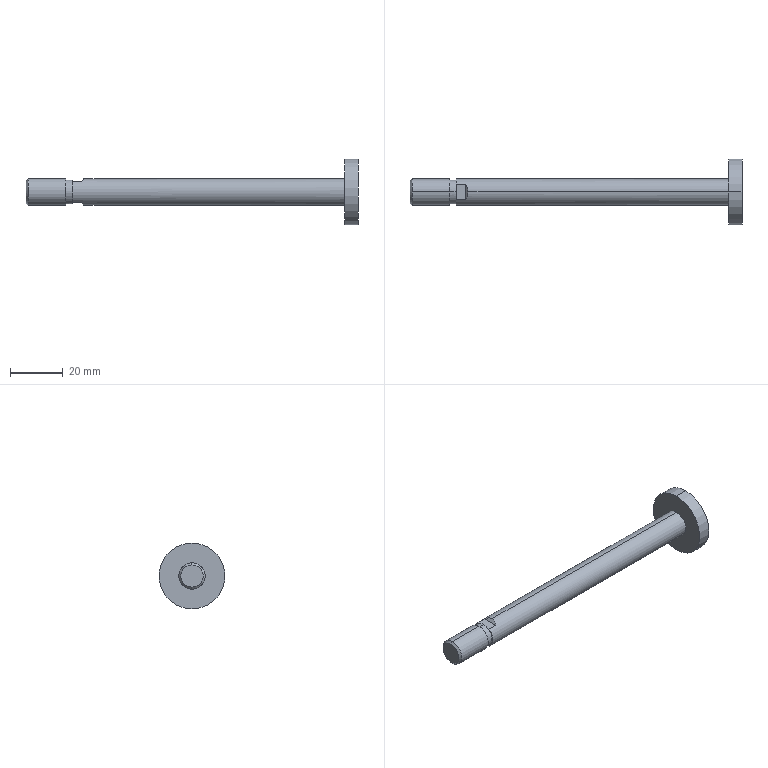Part | SolidWorks | features BaseBody 1 | 1 solid | 22 faces | box 126 x 25 x 25 mm | volume 11883 mm3 | plane 12 | cylinder 8 | cone 2 | commonest cylinder face diameters 10 x4 9.1 x2 25 x2
STEP:
#1=CARTESIAN_POINT('',(21.,3.,4.));
#2=VERTEX_POINT('',#1);
#3=CARTESIAN_POINT('',(22.,0.,5.));
#4=VERTEX_POINT('',#3);
#5=CARTESIAN_POINT('',(21.,3.,4.));
#6=CARTESIAN_POINT('',(21.655,2.127,4.655));
#7=CARTESIAN_POINT('',(22.,1.091,5.));
#8=CARTESIAN_POINT('',(22.,0.,5.));
#9=(BOUNDED_CURVE()B_SPLINE_CURVE(3,(#5,#6,#7,#8),.UNSPECIFIED.,.F.,.T.)B_SPLINE_CURVE_WITH_KNOTS((4,4),(5.64,6.283),.UNSPECIFIED.)CURVE()GEOMETRIC_REPRESENTATION_ITEM()RATIONAL_B_SPLINE_CURVE((1.,0.9658,0.9658,1.))REPRESENTATION_ITEM(''));
#10=EDGE_CURVE('',#2,#4,#9,.T.);
#11=ORIENTED_EDGE('',*,*,#10,.T.);
#12=CARTESIAN_POINT('',(121.,0.,5.));
#13=VERTEX_POINT('',#12);
#14=CARTESIAN_POINT('',(15.,0.,5.));
#15=DIRECTION('',(1.,0.,0.));
#16=VECTOR('',#15,1000.);
#17=LINE('',#14,#16);
#18=EDGE_CURVE('',#4,#13,#17,.T.);
#19=ORIENTED_EDGE('',*,*,#18,.T.);
#20=CARTESIAN_POINT('',(121.,0.,-5.));
#21=VERTEX_POINT('',#20);
#22=CARTESIAN_POINT('',(121.,0.,0.));
#23=DIRECTION('',(-1.,0.,0.));
#24=DIRECTION('',(0.,0.,-1.));
#25=AXIS2_PLACEMENT_3D('',#22,#23,#24);
#26=CIRCLE('',#25,5.);
#27=EDGE_CURVE('',#13,#21,#26,.T.);
#28=ORIENTED_EDGE('',*,*,#27,.T.);
#29=CARTESIAN_POINT('',(22.,0.,-5.));
#30=VERTEX_POINT('',#29);
#31=CARTESIAN_POINT('',(15.,0.,-5.));
#32=DIRECTION('',(1.,0.,0.));
#33=VECTOR('',#32,1000.);
#34=LINE('',#31,#33);
#35=EDGE_CURVE('',#30,#21,#34,.T.);
#36=ORIENTED_EDGE('',*,*,#35,.F.);
#37=CARTESIAN_POINT('',(21.,3.,-4.));
#38=VERTEX_POINT('',#37);
#39=CARTESIAN_POINT('',(22.,0.,-5.));
#40=CARTESIAN_POINT('',(22.,1.091,-5.));
#41=CARTESIAN_POINT('',(21.655,2.127,-4.655));
#42=CARTESIAN_POINT('',(21.,3.,-4.));
#43=(BOUNDED_CURVE()B_SPLINE_CURVE(3,(#39,#40,#41,#42),.UNSPECIFIED.,.F.,.F.)B_SPLINE_CURVE_WITH_KNOTS((4,4),(0.,0.6435),.UNSPECIFIED.)CURVE()GEOMETRIC_REPRESENTATION_ITEM()RATIONAL_B_SPLINE_CURVE((1.,0.9658,0.9658,1.))REPRESENTATION_ITEM(''));
#44=EDGE_CURVE('',#30,#38,#43,.T.);
#45=ORIENTED_EDGE('',*,*,#44,.T.);
#46=CARTESIAN_POINT('',(17.5,3.,-4.));
#47=VERTEX_POINT('',#46);
#48=CARTESIAN_POINT('',(15.,3.,-4.));
#49=DIRECTION('',(-1.,0.,0.));
#50=VECTOR('',#49,1000.);
#51=LINE('',#48,#50);
#52=EDGE_CURVE('',#38,#47,#51,.T.);
#53=ORIENTED_EDGE('',*,*,#52,.T.);
#54=CARTESIAN_POINT('',(17.5,3.,4.));
#55=VERTEX_POINT('',#54);
#56=CARTESIAN_POINT('',(17.5,0.,0.));
#57=DIRECTION('',(1.,0.,0.));
#58=DIRECTION('',(0.,0.,-1.));
#59=AXIS2_PLACEMENT_3D('',#56,#57,#58);
#60=CIRCLE('',#59,5.);
#61=EDGE_CURVE('',#47,#55,#60,.T.);
#62=ORIENTED_EDGE('',*,*,#61,.T.);
#63=CARTESIAN_POINT('',(15.,3.,4.));
#64=DIRECTION('',(1.,0.,0.));
#65=VECTOR('',#64,1000.);
#66=LINE('',#63,#65);
#67=EDGE_CURVE('',#55,#2,#66,.T.);
#68=ORIENTED_EDGE('',*,*,#67,.T.);
#69=EDGE_LOOP('',(#11,#19,#28,#36,#45,#53,#62,#68));
#70=FACE_OUTER_BOUND('',#69,.T.);
#71=CARTESIAN_POINT('',(15.,0.,0.));
#72=DIRECTION('',(1.,0.,0.));
#73=DIRECTION('',(0.,0.,-1.));
#74=AXIS2_PLACEMENT_3D('',#71,#72,#73);
#75=CYLINDRICAL_SURFACE('',#74,5.);
#76=ADVANCED_FACE('',(#70),#75,.T.);
#77=CARTESIAN_POINT('',(15.,0.,-4.55));
#78=VERTEX_POINT('',#77);
#79=CARTESIAN_POINT('',(15.,0.,4.55));
#80=VERTEX_POINT('',#79);
#81=CARTESIAN_POINT('',(15.,0.,0.));
#82=DIRECTION('',(1.,0.,0.));
#83=DIRECTION('',(0.,0.,-1.));
#84=AXIS2_PLACEMENT_3D('',#81,#82,#83);
#85=CIRCLE('',#84,4.55);
#86=EDGE_CURVE('',#78,#80,#85,.T.);
#87=ORIENTED_EDGE('',*,*,#86,.T.);
#88=CARTESIAN_POINT('',(17.5,0.,4.55));
#89=VERTEX_POINT('',#88);
#90=CARTESIAN_POINT('',(15.,0.,4.55));
#91=DIRECTION('',(1.,0.,0.));
#92=VECTOR('',#91,1000.);
#93=LINE('',#90,#92);
#94=EDGE_CURVE('',#80,#89,#93,.T.);
#95=ORIENTED_EDGE('',*,*,#94,.T.);
#96=CARTESIAN_POINT('',(17.5,2.169,4.));
#97=VERTEX_POINT('',#96);
#98=CARTESIAN_POINT('',(17.5,0.,0.));
#99=DIRECTION('',(1.,0.,0.));
#100=DIRECTION('',(0.,0.,-1.));
#101=AXIS2_PLACEMENT_3D('',#98,#99,#100);
#102=CIRCLE('',#101,4.55);
#103=EDGE_CURVE('',#97,#89,#102,.T.);
#104=ORIENTED_EDGE('',*,*,#103,.F.);
#105=CARTESIAN_POINT('',(17.5,2.169,-4.));
#106=VERTEX_POINT('',#105);
#107=CARTESIAN_POINT('',(17.5,0.,0.));
#108=DIRECTION('',(-1.,0.,0.));
#109=DIRECTION('',(0.,0.,-1.));
#110=AXIS2_PLACEMENT_3D('',#107,#108,#109);
#111=CIRCLE('',#110,4.55);
#112=EDGE_CURVE('',#97,#106,#111,.T.);
#113=ORIENTED_EDGE('',*,*,#112,.T.);
#114=CARTESIAN_POINT('',(17.5,0.,-4.55));
#115=VERTEX_POINT('',#114);
#116=CARTESIAN_POINT('',(17.5,0.,0.));
#117=DIRECTION('',(-1.,0.,0.));
#118=DIRECTION('',(0.,0.,-1.));
#119=AXIS2_PLACEMENT_3D('',#116,#117,#118);
#120=CIRCLE('',#119,4.55);
#121=EDGE_CURVE('',#106,#115,#120,.T.);
#122=ORIENTED_EDGE('',*,*,#121,.T.);
#123=CARTESIAN_POINT('',(15.,0.,-4.55));
#124=DIRECTION('',(1.,0.,0.));
#125=VECTOR('',#124,1000.);
#126=LINE('',#123,#125);
#127=EDGE_CURVE('',#78,#115,#126,.T.);
#128=ORIENTED_EDGE('',*,*,#127,.F.);
#129=EDGE_LOOP('',(#87,#95,#104,#113,#122,#128));
#130=FACE_OUTER_BOUND('',#129,.T.);
#131=CARTESIAN_POINT('',(15.,0.,0.));
#132=DIRECTION('',(1.,0.,0.));
#133=DIRECTION('',(0.,0.,-1.));
#134=AXIS2_PLACEMENT_3D('',#131,#132,#133);
#135=CYLINDRICAL_SURFACE('',#134,4.55);
#136=ADVANCED_FACE('',(#130),#135,.T.);
#137=CARTESIAN_POINT('',(121.,0.,-12.5));
#138=VERTEX_POINT('',#137);
#139=CARTESIAN_POINT('',(121.,0.,12.5));
#140=VERTEX_POINT('',#139);
#141=CARTESIAN_POINT('',(121.,0.,0.));
#142=DIRECTION('',(1.,0.,0.));
#143=DIRECTION('',(0.,0.,-1.));
#144=AXIS2_PLACEMENT_3D('',#141,#142,#143);
#145=CIRCLE('',#144,12.5);
#146=EDGE_CURVE('',#138,#140,#145,.T.);
#147=ORIENTED_EDGE('',*,*,#146,.T.);
#148=CARTESIAN_POINT('',(126.,0.,12.5));
#149=VERTEX_POINT('',#148);
#150=CARTESIAN_POINT('',(15.,0.,12.5));
#151=DIRECTION('',(1.,0.,0.));
#152=VECTOR('',#151,1000.);
#153=LINE('',#150,#152);
#154=EDGE_CURVE('',#140,#149,#153,.T.);
#155=ORIENTED_EDGE('',*,*,#154,.T.);
#156=CARTESIAN_POINT('',(126.,0.,-12.5));
#157=VERTEX_POINT('',#156);
#158=CARTESIAN_POINT('',(126.,0.,0.));
#159=DIRECTION('',(-1.,0.,0.));
#160=DIRECTION('',(0.,0.,-1.));
#161=AXIS2_PLACEMENT_3D('',#158,#159,#160);
#162=CIRCLE('',#161,12.5);
#163=EDGE_CURVE('',#149,#157,#162,.T.);
#164=ORIENTED_EDGE('',*,*,#163,.T.);
#165=CARTESIAN_POINT('',(15.,0.,-12.5));
#166=DIRECTION('',(1.,0.,0.));
#167=VECTOR('',#166,1000.);
#168=LINE('',#165,#167);
#169=EDGE_CURVE('',#138,#157,#168,.T.);
#170=ORIENTED_EDGE('',*,*,#169,.F.);
#171=EDGE_LOOP('',(#147,#155,#164,#170));
#172=FACE_OUTER_BOUND('',#171,.T.);
#173=CARTESIAN_POINT('',(15.,0.,0.));
#174=DIRECTION('',(1.,0.,0.));
#175=DIRECTION('',(0.,0.,-1.));
#176=AXIS2_PLACEMENT_3D('',#173,#174,#175);
#177=CYLINDRICAL_SURFACE('',#176,12.5);
#178=ADVANCED_FACE('',(#172),#177,.T.);
#179=CARTESIAN_POINT('',(0.767,0.,-5.));
#180=VERTEX_POINT('',#179);
#181=CARTESIAN_POINT('',(0.767,0.,5.));
#182=VERTEX_POINT('',#181);
#183=CARTESIAN_POINT('',(0.767,0.,0.));
#184=DIRECTION('',(1.,0.,0.));
#185=DIRECTION('',(0.,0.,-1.));
#186=AXIS2_PLACEMENT_3D('',#183,#184,#185);
#187=CIRCLE('',#186,5.);
#188=EDGE_CURVE('',#180,#182,#187,.T.);
#189=ORIENTED_EDGE('',*,*,#188,.T.);
#190=CARTESIAN_POINT('',(15.,0.,5.));
#191=VERTEX_POINT('',#190);
#192=CARTESIAN_POINT('',(15.,0.,5.));
#193=DIRECTION('',(1.,0.,0.));
#194=VECTOR('',#193,1000.);
#195=LINE('',#192,#194);
#196=EDGE_CURVE('',#182,#191,#195,.T.);
#197=ORIENTED_EDGE('',*,*,#196,.T.);
#198=CARTESIAN_POINT('',(15.,0.,-5.));
#199=VERTEX_POINT('',#198);
#200=CARTESIAN_POINT('',(15.,0.,0.));
#201=DIRECTION('',(-1.,0.,0.));
#202=DIRECTION('',(0.,0.,-1.));
#203=AXIS2_PLACEMENT_3D('',#200,#201,#202);
#204=CIRCLE('',#203,5.);
#205=EDGE_CURVE('',#191,#199,#204,.T.);
#206=ORIENTED_EDGE('',*,*,#205,.T.);
#207=CARTESIAN_POINT('',(15.,0.,-5.));
#208=DIRECTION('',(1.,0.,0.));
#209=VECTOR('',#208,1000.);
#210=LINE('',#207,#209);
#211=EDGE_CURVE('',#180,#199,#210,.T.);
#212=ORIENTED_EDGE('',*,*,#211,.F.);
#213=EDGE_LOOP('',(#189,#197,#206,#212));
#214=FACE_OUTER_BOUND('',#213,.T.);
#215=CARTESIAN_POINT('',(15.,0.,0.));
#216=DIRECTION('',(1.,0.,0.));
#217=DIRECTION('',(0.,0.,-1.));
#218=AXIS2_PLACEMENT_3D('',#215,#216,#217);
#219=CYLINDRICAL_SURFACE('',#218,5.);
#220=ADVANCED_FACE('',(#214),#219,.T.);
#221=CARTESIAN_POINT('',(0.,0.,-4.233));
#222=VERTEX_POINT('',#221);
#223=CARTESIAN_POINT('',(0.,0.,4.233));
#224=VERTEX_POINT('',#223);
#225=CARTESIAN_POINT('',(0.,0.,0.));
#226=DIRECTION('',(1.,0.,0.));
#227=DIRECTION('',(0.,0.,-1.));
#228=AXIS2_PLACEMENT_3D('',#225,#226,#227);
#229=CIRCLE('',#228,4.233);
#230=EDGE_CURVE('',#222,#224,#229,.T.);
#231=ORIENTED_EDGE('',*,*,#230,.T.);
#232=CARTESIAN_POINT('',(0.767,0.,5.));
#233=DIRECTION('',(0.7071,0.,0.7071));
#234=VECTOR('',#233,1000.);
#235=LINE('',#232,#234);
#236=EDGE_CURVE('',#224,#182,#235,.T.);
#237=ORIENTED_EDGE('',*,*,#236,.T.);
#238=ORIENTED_EDGE('',*,*,#188,.F.);
#239=CARTESIAN_POINT('',(0.767,0.,-5.));
#240=DIRECTION('',(0.7071,0.,-0.7071));
#241=VECTOR('',#240,1000.);
#242=LINE('',#239,#241);
#243=EDGE_CURVE('',#222,#180,#242,.T.);
#244=ORIENTED_EDGE('',*,*,#243,.F.);
#245=EDGE_LOOP('',(#231,#237,#238,#244));
#246=FACE_OUTER_BOUND('',#245,.T.);
#247=CARTESIAN_POINT('',(0.767,0.,0.));
#248=DIRECTION('',(1.,0.,0.));
#249=DIRECTION('',(0.,0.,-1.));
#250=AXIS2_PLACEMENT_3D('',#247,#248,#249);
#251=CONICAL_SURFACE('',#250,5.,0.7854);
#252=ADVANCED_FACE('',(#246),#251,.T.);
#253=ORIENTED_EDGE('',*,*,#18,.F.);
#254=CARTESIAN_POINT('',(21.,-3.,4.));
#255=VERTEX_POINT('',#254);
#256=CARTESIAN_POINT('',(22.,0.,5.));
#257=CARTESIAN_POINT('',(22.,-1.091,5.));
#258=CARTESIAN_POINT('',(21.655,-2.127,4.655));
#259=CARTESIAN_POINT('',(21.,-3.,4.));
#260=(BOUNDED_CURVE()B_SPLINE_CURVE(3,(#256,#257,#258,#259),.UNSPECIFIED.,.F.,.F.)B_SPLINE_CURVE_WITH_KNOTS((4,4),(0.,0.6435),.UNSPECIFIED.)CURVE()GEOMETRIC_REPRESENTATION_ITEM()RATIONAL_B_SPLINE_CURVE((1.,0.9658,0.9658,1.))REPRESENTATION_ITEM(''));
#261=EDGE_CURVE('',#4,#255,#260,.T.);
#262=ORIENTED_EDGE('',*,*,#261,.T.);
#263=CARTESIAN_POINT('',(17.5,-3.,4.));
#264=VERTEX_POINT('',#263);
#265=CARTESIAN_POINT('',(15.,-3.,4.));
#266=DIRECTION('',(-1.,0.,0.));
#267=VECTOR('',#266,1000.);
#268=LINE('',#265,#267);
#269=EDGE_CURVE('',#255,#264,#268,.T.);
#270=ORIENTED_EDGE('',*,*,#269,.T.);
#271=CARTESIAN_POINT('',(17.5,-3.,-4.));
#272=VERTEX_POINT('',#271);
#273=CARTESIAN_POINT('',(17.5,0.,0.));
#274=DIRECTION('',(1.,0.,0.));
#275=DIRECTION('',(0.,0.,-1.));
#276=AXIS2_PLACEMENT_3D('',#273,#274,#275);
#277=CIRCLE('',#276,5.);
#278=EDGE_CURVE('',#264,#272,#277,.T.);
#279=ORIENTED_EDGE('',*,*,#278,.T.);
#280=CARTESIAN_POINT('',(21.,-3.,-4.));
#281=VERTEX_POINT('',#280);
#282=CARTESIAN_POINT('',(15.,-3.,-4.));
#283=DIRECTION('',(1.,0.,0.));
#284=VECTOR('',#283,1000.);
#285=LINE('',#282,#284);
#286=EDGE_CURVE('',#272,#281,#285,.T.);
#287=ORIENTED_EDGE('',*,*,#286,.T.);
#288=CARTESIAN_POINT('',(21.,-3.,-4.));
#289=CARTESIAN_POINT('',(21.655,-2.127,-4.655));
#290=CARTESIAN_POINT('',(22.,-1.091,-5.));
#291=CARTESIAN_POINT('',(22.,0.,-5.));
#292=(BOUNDED_CURVE()B_SPLINE_CURVE(3,(#288,#289,#290,#291),.UNSPECIFIED.,.F.,.F.)B_SPLINE_CURVE_WITH_KNOTS((4,4),(5.64,6.283),.UNSPECIFIED.)CURVE()GEOMETRIC_REPRESENTATION_ITEM()RATIONAL_B_SPLINE_CURVE((1.,0.9658,0.9658,1.))REPRESENTATION_ITEM(''));
#293=EDGE_CURVE('',#281,#30,#292,.T.);
#294=ORIENTED_EDGE('',*,*,#293,.T.);
#295=ORIENTED_EDGE('',*,*,#35,.T.);
#296=CARTESIAN_POINT('',(121.,0.,0.));
#297=DIRECTION('',(-1.,0.,0.));
#298=DIRECTION('',(0.,0.,-1.));
#299=AXIS2_PLACEMENT_3D('',#296,#297,#298);
#300=CIRCLE('',#299,5.);
#301=EDGE_CURVE('',#21,#13,#300,.T.);
#302=ORIENTED_EDGE('',*,*,#301,.T.);
#303=EDGE_LOOP('',(#253,#262,#270,#279,#287,#294,#295,#302));
#304=FACE_OUTER_BOUND('',#303,.T.);
#305=CARTESIAN_POINT('',(15.,0.,0.));
#306=DIRECTION('',(1.,0.,0.));
#307=DIRECTION('',(0.,0.,-1.));
#308=AXIS2_PLACEMENT_3D('',#305,#306,#307);
#309=CYLINDRICAL_SURFACE('',#308,5.);
#310=ADVANCED_FACE('',(#304),#309,.T.);
#311=ORIENTED_EDGE('',*,*,#10,.F.);
#312=CARTESIAN_POINT('',(21.,5.,4.));
#313=DIRECTION('',(0.,-1.,0.));
#314=VECTOR('',#313,1000.);
#315=LINE('',#312,#314);
#316=EDGE_CURVE('',#2,#255,#315,.T.);
#317=ORIENTED_EDGE('',*,*,#316,.T.);
#318=ORIENTED_EDGE('',*,*,#261,.F.);
#319=EDGE_LOOP('',(#311,#317,#318));
#320=FACE_OUTER_BOUND('',#319,.T.);
#321=CARTESIAN_POINT('',(26.,5.,9.));
#322=DIRECTION('',(-0.7071,0.,0.7071));
#323=DIRECTION('',(0.7071,0.,0.7071));
#324=AXIS2_PLACEMENT_3D('',#321,#322,#323);
#325=PLANE('',#324);
#326=ADVANCED_FACE('',(#320),#325,.T.);
#327=CARTESIAN_POINT('',(17.5,-2.169,4.));
#328=VERTEX_POINT('',#327);
#329=CARTESIAN_POINT('',(17.5,5.,4.));
#330=DIRECTION('',(0.,-1.,0.));
#331=VECTOR('',#330,1000.);
#332=LINE('',#329,#331);
#333=EDGE_CURVE('',#97,#328,#332,.T.);
#334=ORIENTED_EDGE('',*,*,#333,.T.);
#335=CARTESIAN_POINT('',(17.5,5.,4.));
#336=DIRECTION('',(0.,-1.,0.));
#337=VECTOR('',#336,1000.);
#338=LINE('',#335,#337);
#339=EDGE_CURVE('',#328,#264,#338,.T.);
#340=ORIENTED_EDGE('',*,*,#339,.T.);
#341=ORIENTED_EDGE('',*,*,#269,.F.);
#342=ORIENTED_EDGE('',*,*,#316,.F.);
#343=ORIENTED_EDGE('',*,*,#67,.F.);
#344=CARTESIAN_POINT('',(17.5,5.,4.));
#345=DIRECTION('',(0.,-1.,0.));
#346=VECTOR('',#345,1000.);
#347=LINE('',#344,#346);
#348=EDGE_CURVE('',#55,#97,#347,.T.);
#349=ORIENTED_EDGE('',*,*,#348,.T.);
#350=EDGE_LOOP('',(#334,#340,#341,#342,#343,#349));
#351=FACE_OUTER_BOUND('',#350,.T.);
#352=CARTESIAN_POINT('',(21.,5.,4.));
#353=DIRECTION('',(0.,0.,1.));
#354=DIRECTION('',(1.,0.,0.));
#355=AXIS2_PLACEMENT_3D('',#352,#353,#354);
#356=PLANE('',#355);
#357=ADVANCED_FACE('',(#351),#356,.T.);
#358=ORIENTED_EDGE('',*,*,#61,.F.);
#359=CARTESIAN_POINT('',(17.5,4.55,-4.));
#360=DIRECTION('',(0.,1.,0.));
#361=VECTOR('',#360,1000.);
#362=LINE('',#359,#361);
#363=EDGE_CURVE('',#106,#47,#362,.T.);
#364=ORIENTED_EDGE('',*,*,#363,.F.);
#365=ORIENTED_EDGE('',*,*,#112,.F.);
#366=ORIENTED_EDGE('',*,*,#348,.F.);
#367=EDGE_LOOP('',(#358,#364,#365,#366));
#368=FACE_OUTER_BOUND('',#367,.T.);
#369=CARTESIAN_POINT('',(17.5,4.55,0.));
#370=DIRECTION('',(1.,0.,0.));
#371=DIRECTION('',(0.,0.,-1.));
#372=AXIS2_PLACEMENT_3D('',#369,#370,#371);
#373=PLANE('',#372);
#374=ADVANCED_FACE('',(#368),#373,.F.);
#375=CARTESIAN_POINT('',(17.5,-2.169,-4.));
#376=VERTEX_POINT('',#375);
#377=CARTESIAN_POINT('',(17.5,5.,-4.));
#378=DIRECTION('',(0.,1.,0.));
#379=VECTOR('',#378,1000.);
#380=LINE('',#377,#379);
#381=EDGE_CURVE('',#376,#106,#380,.T.);
#382=ORIENTED_EDGE('',*,*,#381,.T.);
#383=ORIENTED_EDGE('',*,*,#363,.T.);
#384=ORIENTED_EDGE('',*,*,#52,.F.);
#385=CARTESIAN_POINT('',(21.,5.,-4.));
#386=DIRECTION('',(0.,-1.,0.));
#387=VECTOR('',#386,1000.);
#388=LINE('',#385,#387);
#389=EDGE_CURVE('',#38,#281,#388,.T.);
#390=ORIENTED_EDGE('',*,*,#389,.T.);
#391=ORIENTED_EDGE('',*,*,#286,.F.);
#392=CARTESIAN_POINT('',(17.5,5.,-4.));
#393=DIRECTION('',(0.,1.,0.));
#394=VECTOR('',#393,1000.);
#395=LINE('',#392,#394);
#396=EDGE_CURVE('',#272,#376,#395,.T.);
#397=ORIENTED_EDGE('',*,*,#396,.T.);
#398=EDGE_LOOP('',(#382,#383,#384,#390,#391,#397));
#399=FACE_OUTER_BOUND('',#398,.T.);
#400=CARTESIAN_POINT('',(17.5,5.,-4.));
#401=DIRECTION('',(0.,0.,-1.));
#402=DIRECTION('',(-1.,0.,0.));
#403=AXIS2_PLACEMENT_3D('',#400,#401,#402);
#404=PLANE('',#403);
#405=ADVANCED_FACE('',(#399),#404,.T.);
#406=ORIENTED_EDGE('',*,*,#293,.F.);
#407=ORIENTED_EDGE('',*,*,#389,.F.);
#408=ORIENTED_EDGE('',*,*,#44,.F.);
#409=EDGE_LOOP('',(#406,#407,#408));
#410=FACE_OUTER_BOUND('',#409,.T.);
#411=CARTESIAN_POINT('',(21.,5.,-4.));
#412=DIRECTION('',(-0.7071,0.,-0.7071));
#413=DIRECTION('',(-0.7071,0.,0.7071));
#414=AXIS2_PLACEMENT_3D('',#411,#412,#413);
#415=PLANE('',#414);
#416=ADVANCED_FACE('',(#410),#415,.T.);
#417=CARTESIAN_POINT('',(17.5,0.,0.));
#418=DIRECTION('',(-1.,0.,0.));
#419=DIRECTION('',(0.,0.,-1.));
#420=AXIS2_PLACEMENT_3D('',#417,#418,#419);
#421=CIRCLE('',#420,4.55);
#422=EDGE_CURVE('',#376,#328,#421,.T.);
#423=ORIENTED_EDGE('',*,*,#422,.F.);
#424=ORIENTED_EDGE('',*,*,#396,.F.);
#425=ORIENTED_EDGE('',*,*,#278,.F.);
#426=ORIENTED_EDGE('',*,*,#339,.F.);
#427=EDGE_LOOP('',(#423,#424,#425,#426));
#428=FACE_OUTER_BOUND('',#427,.T.);
#429=CARTESIAN_POINT('',(17.5,4.55,0.));
#430=DIRECTION('',(1.,0.,0.));
#431=DIRECTION('',(0.,0.,-1.));
#432=AXIS2_PLACEMENT_3D('',#429,#430,#431);
#433=PLANE('',#432);
#434=ADVANCED_FACE('',(#428),#433,.F.);
#435=ORIENTED_EDGE('',*,*,#301,.F.);
#436=ORIENTED_EDGE('',*,*,#27,.F.);
#437=EDGE_LOOP('',(#435,#436));
#438=FACE_BOUND('',#437,.T.);
#439=ORIENTED_EDGE('',*,*,#146,.F.);
#440=CARTESIAN_POINT('',(121.,0.,0.));
#441=DIRECTION('',(1.,0.,0.));
#442=DIRECTION('',(0.,0.,-1.));
#443=AXIS2_PLACEMENT_3D('',#440,#441,#442);
#444=CIRCLE('',#443,12.5);
#445=EDGE_CURVE('',#140,#138,#444,.T.);
#446=ORIENTED_EDGE('',*,*,#445,.F.);
#447=EDGE_LOOP('',(#439,#446));
#448=FACE_OUTER_BOUND('',#447,.T.);
#449=CARTESIAN_POINT('',(121.,5.,0.));
#450=DIRECTION('',(1.,0.,0.));
#451=DIRECTION('',(0.,0.,-1.));
#452=AXIS2_PLACEMENT_3D('',#449,#450,#451);
#453=PLANE('',#452);
#454=ADVANCED_FACE('',(#438,#448),#453,.F.);
#455=ORIENTED_EDGE('',*,*,#103,.T.);
#456=CARTESIAN_POINT('',(17.5,0.,0.));
#457=DIRECTION('',(1.,0.,0.));
#458=DIRECTION('',(0.,0.,-1.));
#459=AXIS2_PLACEMENT_3D('',#456,#457,#458);
#460=CIRCLE('',#459,4.55);
#461=EDGE_CURVE('',#89,#328,#460,.T.);
#462=ORIENTED_EDGE('',*,*,#461,.T.);
#463=ORIENTED_EDGE('',*,*,#333,.F.);
#464=EDGE_LOOP('',(#455,#462,#463));
#465=FACE_OUTER_BOUND('',#464,.T.);
#466=CARTESIAN_POINT('',(17.5,5.,4.));
#467=DIRECTION('',(1.,0.,0.));
#468=DIRECTION('',(0.,0.,-1.));
#469=AXIS2_PLACEMENT_3D('',#466,#467,#468);
#470=PLANE('',#469);
#471=ADVANCED_FACE('',(#465),#470,.T.);
#472=ORIENTED_EDGE('',*,*,#94,.F.);
#473=CARTESIAN_POINT('',(15.,0.,0.));
#474=DIRECTION('',(1.,0.,0.));
#475=DIRECTION('',(0.,0.,-1.));
#476=AXIS2_PLACEMENT_3D('',#473,#474,#475);
#477=CIRCLE('',#476,4.55);
#478=EDGE_CURVE('',#80,#78,#477,.T.);
#479=ORIENTED_EDGE('',*,*,#478,.T.);
#480=ORIENTED_EDGE('',*,*,#127,.T.);
#481=CARTESIAN_POINT('',(17.5,0.,0.));
#482=DIRECTION('',(-1.,0.,0.));
#483=DIRECTION('',(0.,0.,-1.));
#484=AXIS2_PLACEMENT_3D('',#481,#482,#483);
#485=CIRCLE('',#484,4.55);
#486=EDGE_CURVE('',#115,#376,#485,.T.);
#487=ORIENTED_EDGE('',*,*,#486,.T.);
#488=ORIENTED_EDGE('',*,*,#422,.T.);
#489=ORIENTED_EDGE('',*,*,#461,.F.);
#490=EDGE_LOOP('',(#472,#479,#480,#487,#488,#489));
#491=FACE_OUTER_BOUND('',#490,.T.);
#492=CARTESIAN_POINT('',(15.,0.,0.));
#493=DIRECTION('',(1.,0.,0.));
#494=DIRECTION('',(0.,0.,-1.));
#495=AXIS2_PLACEMENT_3D('',#492,#493,#494);
#496=CYLINDRICAL_SURFACE('',#495,4.55);
#497=ADVANCED_FACE('',(#491),#496,.T.);
#498=ORIENTED_EDGE('',*,*,#121,.F.);
#499=ORIENTED_EDGE('',*,*,#381,.F.);
#500=ORIENTED_EDGE('',*,*,#486,.F.);
#501=EDGE_LOOP('',(#498,#499,#500));
#502=FACE_OUTER_BOUND('',#501,.T.);
#503=CARTESIAN_POINT('',(17.5,5.,-9.));
#504=DIRECTION('',(1.,0.,0.));
#505=DIRECTION('',(0.,0.,-1.));
#506=AXIS2_PLACEMENT_3D('',#503,#504,#505);
#507=PLANE('',#506);
#508=ADVANCED_FACE('',(#502),#507,.T.);
#509=ORIENTED_EDGE('',*,*,#154,.F.);
#510=ORIENTED_EDGE('',*,*,#445,.T.);
#511=ORIENTED_EDGE('',*,*,#169,.T.);
#512=CARTESIAN_POINT('',(126.,0.,0.));
#513=DIRECTION('',(-1.,0.,0.));
#514=DIRECTION('',(0.,0.,-1.));
#515=AXIS2_PLACEMENT_3D('',#512,#513,#514);
#516=CIRCLE('',#515,12.5);
#517=EDGE_CURVE('',#157,#149,#516,.T.);
#518=ORIENTED_EDGE('',*,*,#517,.T.);
#519=EDGE_LOOP('',(#509,#510,#511,#518));
#520=FACE_OUTER_BOUND('',#519,.T.);
#521=CARTESIAN_POINT('',(15.,0.,0.));
#522=DIRECTION('',(1.,0.,0.));
#523=DIRECTION('',(0.,0.,-1.));
#524=AXIS2_PLACEMENT_3D('',#521,#522,#523);
#525=CYLINDRICAL_SURFACE('',#524,12.5);
#526=ADVANCED_FACE('',(#520),#525,.T.);
#527=CARTESIAN_POINT('',(15.,0.,0.));
#528=DIRECTION('',(-1.,0.,0.));
#529=DIRECTION('',(0.,0.,-1.));
#530=AXIS2_PLACEMENT_3D('',#527,#528,#529);
#531=CIRCLE('',#530,5.);
#532=EDGE_CURVE('',#199,#191,#531,.T.);
#533=ORIENTED_EDGE('',*,*,#532,.F.);
#534=ORIENTED_EDGE('',*,*,#205,.F.);
#535=EDGE_LOOP('',(#533,#534));
#536=FACE_OUTER_BOUND('',#535,.T.);
#537=ORIENTED_EDGE('',*,*,#86,.F.);
#538=ORIENTED_EDGE('',*,*,#478,.F.);
#539=EDGE_LOOP('',(#537,#538));
#540=FACE_BOUND('',#539,.T.);
#541=CARTESIAN_POINT('',(15.,5.,0.));
#542=DIRECTION('',(-1.,0.,0.));
#543=DIRECTION('',(0.,0.,1.));
#544=AXIS2_PLACEMENT_3D('',#541,#542,#543);
#545=PLANE('',#544);
#546=ADVANCED_FACE('',(#536,#540),#545,.F.);
#547=ORIENTED_EDGE('',*,*,#517,.F.);
#548=ORIENTED_EDGE('',*,*,#163,.F.);
#549=EDGE_LOOP('',(#547,#548));
#550=FACE_OUTER_BOUND('',#549,.T.);
#551=CARTESIAN_POINT('',(126.,12.5,0.));
#552=DIRECTION('',(-1.,0.,0.));
#553=DIRECTION('',(0.,0.,1.));
#554=AXIS2_PLACEMENT_3D('',#551,#552,#553);
#555=PLANE('',#554);
#556=ADVANCED_FACE('',(#550),#555,.F.);
#557=ORIENTED_EDGE('',*,*,#196,.F.);
#558=CARTESIAN_POINT('',(0.767,0.,0.));
#559=DIRECTION('',(1.,0.,0.));
#560=DIRECTION('',(0.,0.,-1.));
#561=AXIS2_PLACEMENT_3D('',#558,#559,#560);
#562=CIRCLE('',#561,5.);
#563=EDGE_CURVE('',#182,#180,#562,.T.);
#564=ORIENTED_EDGE('',*,*,#563,.T.);
#565=ORIENTED_EDGE('',*,*,#211,.T.);
#566=ORIENTED_EDGE('',*,*,#532,.T.);
#567=EDGE_LOOP('',(#557,#564,#565,#566));
#568=FACE_OUTER_BOUND('',#567,.T.);
#569=CARTESIAN_POINT('',(15.,0.,0.));
#570=DIRECTION('',(1.,0.,0.));
#571=DIRECTION('',(0.,0.,-1.));
#572=AXIS2_PLACEMENT_3D('',#569,#570,#571);
#573=CYLINDRICAL_SURFACE('',#572,5.);
#574=ADVANCED_FACE('',(#568),#573,.T.);
#575=ORIENTED_EDGE('',*,*,#236,.F.);
#576=CARTESIAN_POINT('',(0.,0.,0.));
#577=DIRECTION('',(1.,0.,0.));
#578=DIRECTION('',(0.,0.,-1.));
#579=AXIS2_PLACEMENT_3D('',#576,#577,#578);
#580=CIRCLE('',#579,4.233);
#581=EDGE_CURVE('',#224,#222,#580,.T.);
#582=ORIENTED_EDGE('',*,*,#581,.T.);
#583=ORIENTED_EDGE('',*,*,#243,.T.);
#584=ORIENTED_EDGE('',*,*,#563,.F.);
#585=EDGE_LOOP('',(#575,#582,#583,#584));
#586=FACE_OUTER_BOUND('',#585,.T.);
#587=CARTESIAN_POINT('',(0.767,0.,0.));
#588=DIRECTION('',(1.,0.,0.));
#589=DIRECTION('',(0.,0.,-1.));
#590=AXIS2_PLACEMENT_3D('',#587,#588,#589);
#591=CONICAL_SURFACE('',#590,5.,0.7854);
#592=ADVANCED_FACE('',(#586),#591,.T.);
#593=ORIENTED_EDGE('',*,*,#230,.F.);
#594=ORIENTED_EDGE('',*,*,#581,.F.);
#595=EDGE_LOOP('',(#593,#594));
#596=FACE_OUTER_BOUND('',#595,.T.);
#597=CARTESIAN_POINT('',(0.,0.,0.));
#598=DIRECTION('',(1.,0.,0.));
#599=DIRECTION('',(0.,0.,-1.));
#600=AXIS2_PLACEMENT_3D('',#597,#598,#599);
#601=PLANE('',#600);
#602=ADVANCED_FACE('',(#596),#601,.F.);
#603=CLOSED_SHELL('',(#76,#136,#178,#220,#252,#310,#326,#357,#374,#405,#416,#434,#454,#471,#497,#508,#526,#546,#556,#574,#592,#602));
#604=MANIFOLD_SOLID_BREP('',#603);
#605=CARTESIAN_POINT('',(0.,0.,0.));
#606=DIRECTION('',(0.,0.,1.));
#607=DIRECTION('',(1.,0.,0.));
#608=AXIS2_PLACEMENT_3D('',#605,#606,#607);
#609=(LENGTH_UNIT()NAMED_UNIT(*)SI_UNIT(.MILLI.,.METRE.));
#610=UNCERTAINTY_MEASURE_WITH_UNIT(LENGTH_MEASURE(0.00001),#609,'','');
#611=(NAMED_UNIT(*)PLANE_ANGLE_UNIT()SI_UNIT($,.RADIAN.));
#612=(NAMED_UNIT(*)SI_UNIT($,.STERADIAN.)SOLID_ANGLE_UNIT());
#613=(GEOMETRIC_REPRESENTATION_CONTEXT(3)GLOBAL_UNCERTAINTY_ASSIGNED_CONTEXT((#610))GLOBAL_UNIT_ASSIGNED_CONTEXT((#609,#611,#612))REPRESENTATION_CONTEXT('',''));
#614=ADVANCED_BREP_SHAPE_REPRESENTATION('',(#604,#608),#613);